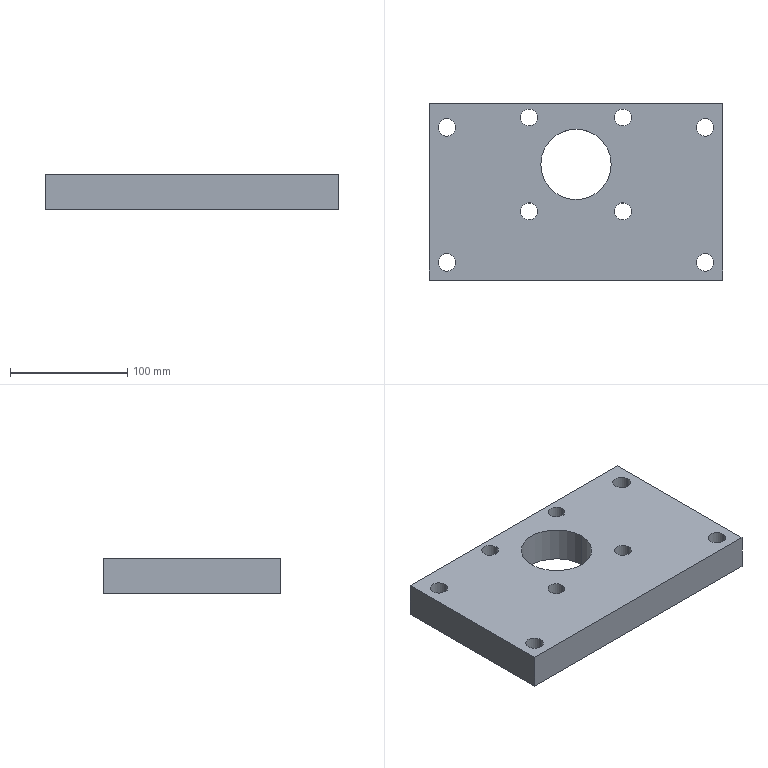Part | STEP file | TAM GA XYLANH GIUA | 1 solid | 24 faces | box 250 x 150 x 30 mm | volume 999493 mm3 | cylinder 18 | plane 6 | commonest cylinder face diameters 14.376 x8 15 x8 60 x2